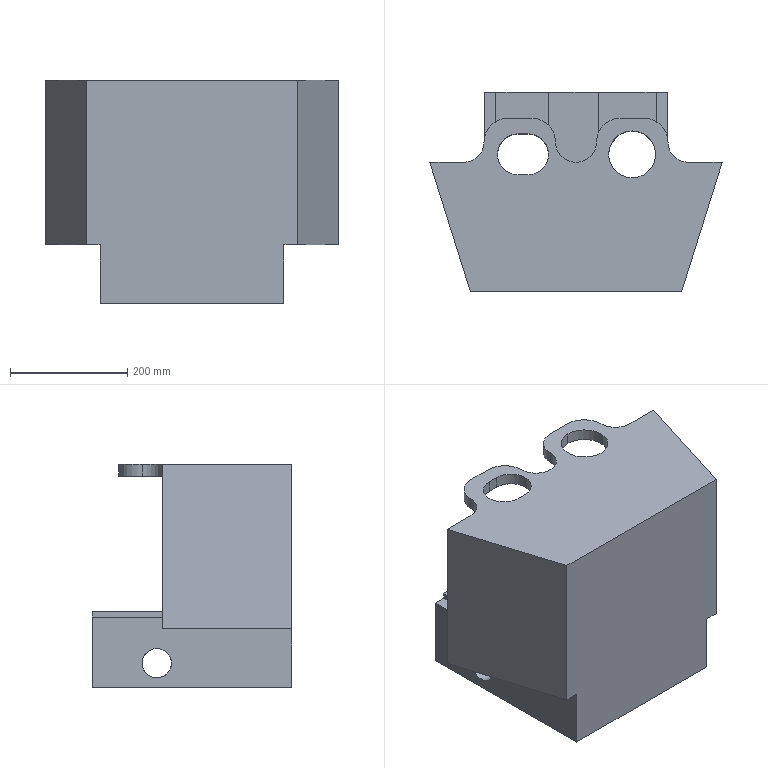Part | SolidWorks | features ICE 7, 3DProfileFeature 6, BlendCut 1, Extrusion 1, MirrorPattern 1 | 1 solid | 52 faces | box 498.198 x 340 x 380 mm | volume 18859661 mm3 | plane 31 | cylinder 21 | commonest cylinder face diameters 80 x8 70 x7 50 x6